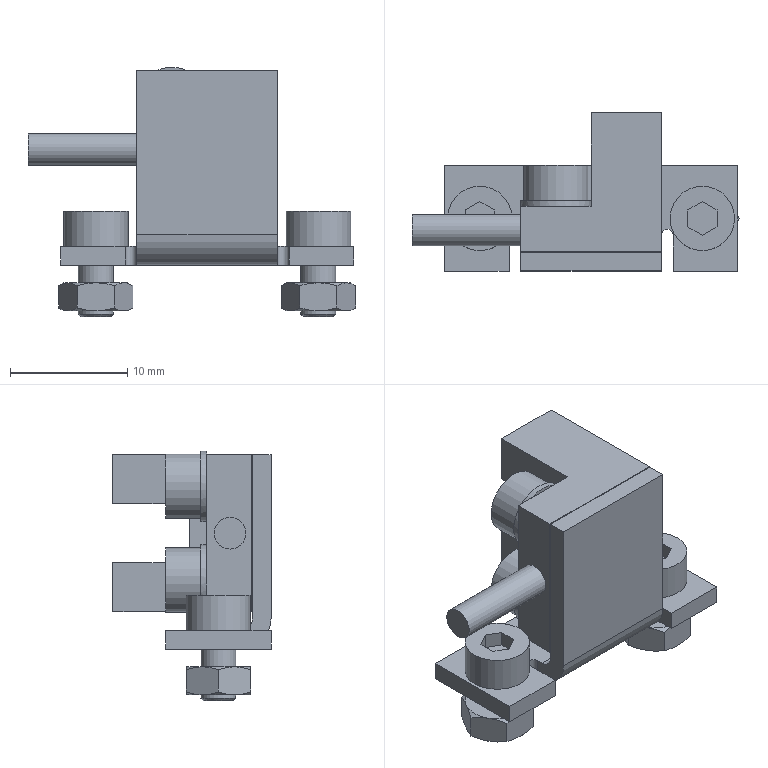Part | STEP file | LX_SENSOR_SET-EP | 1 solid | 130 faces | box 27.925 x 13.5 x 21.3 mm | volume 2192 mm3 | plane 89 | cone 26 | cylinder 15 | commonest cylinder face diameters 3 x4 5.5 x4 1 x2 6 x2 2 x1 2.7 x1